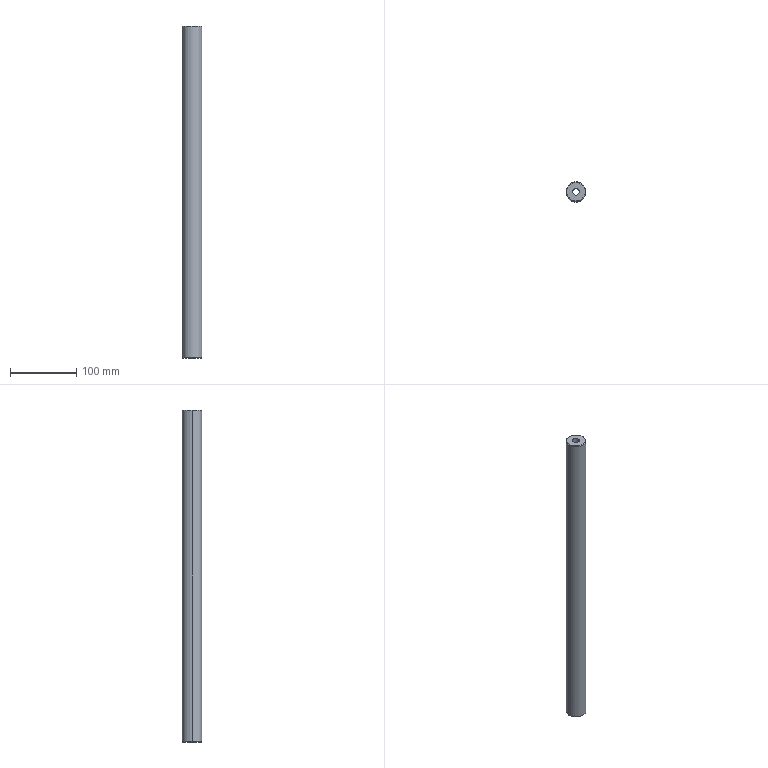Part | SolidWorks | features BaseBody 1 | 1 solid | 10 faces | box 30 x 30 x 500 mm | volume 312481 mm3 | cone 4 | cylinder 4 | plane 2 | commonest cylinder face diameters 10.2 x2 30 x2
STEP:
#1=CARTESIAN_POINT('',(14.,0.,500.));
#2=VERTEX_POINT('',#1);
#3=CARTESIAN_POINT('',(-14.,0.,500.));
#4=VERTEX_POINT('',#3);
#5=CARTESIAN_POINT('',(0.,0.,500.));
#6=DIRECTION('',(0.,0.,1.));
#7=DIRECTION('',(-1.,0.,0.));
#8=AXIS2_PLACEMENT_3D('',#5,#6,#7);
#9=CIRCLE('',#8,14.);
#10=EDGE_CURVE('',#2,#4,#9,.T.);
#11=ORIENTED_EDGE('',*,*,#10,.F.);
#12=CARTESIAN_POINT('',(15.,0.,499.));
#13=VERTEX_POINT('',#12);
#14=CARTESIAN_POINT('',(14.,0.,500.));
#15=DIRECTION('',(0.7071,0.,-0.7071));
#16=VECTOR('',#15,1000.);
#17=LINE('',#14,#16);
#18=EDGE_CURVE('',#2,#13,#17,.T.);
#19=ORIENTED_EDGE('',*,*,#18,.T.);
#20=CARTESIAN_POINT('',(-15.,0.,499.));
#21=VERTEX_POINT('',#20);
#22=CARTESIAN_POINT('',(0.,0.,499.));
#23=DIRECTION('',(0.,0.,-1.));
#24=DIRECTION('',(-1.,0.,0.));
#25=AXIS2_PLACEMENT_3D('',#22,#23,#24);
#26=CIRCLE('',#25,15.);
#27=EDGE_CURVE('',#21,#13,#26,.T.);
#28=ORIENTED_EDGE('',*,*,#27,.F.);
#29=CARTESIAN_POINT('',(-14.,0.,500.));
#30=DIRECTION('',(-0.7071,0.,-0.7071));
#31=VECTOR('',#30,1000.);
#32=LINE('',#29,#31);
#33=EDGE_CURVE('',#4,#21,#32,.T.);
#34=ORIENTED_EDGE('',*,*,#33,.F.);
#35=EDGE_LOOP('',(#11,#19,#28,#34));
#36=FACE_OUTER_BOUND('',#35,.T.);
#37=CARTESIAN_POINT('',(0.,0.,500.));
#38=DIRECTION('',(0.,0.,-1.));
#39=DIRECTION('',(-1.,0.,0.));
#40=AXIS2_PLACEMENT_3D('',#37,#38,#39);
#41=CONICAL_SURFACE('',#40,14.,0.7854);
#42=ADVANCED_FACE('',(#36),#41,.T.);
#43=ORIENTED_EDGE('',*,*,#27,.T.);
#44=CARTESIAN_POINT('',(15.,0.,1.));
#45=VERTEX_POINT('',#44);
#46=CARTESIAN_POINT('',(15.,0.,499.));
#47=DIRECTION('',(0.,0.,-1.));
#48=VECTOR('',#47,1000.);
#49=LINE('',#46,#48);
#50=EDGE_CURVE('',#13,#45,#49,.T.);
#51=ORIENTED_EDGE('',*,*,#50,.T.);
#52=CARTESIAN_POINT('',(-15.,0.,1.));
#53=VERTEX_POINT('',#52);
#54=CARTESIAN_POINT('',(0.,0.,1.));
#55=DIRECTION('',(0.,0.,-1.));
#56=DIRECTION('',(-1.,0.,0.));
#57=AXIS2_PLACEMENT_3D('',#54,#55,#56);
#58=CIRCLE('',#57,15.);
#59=EDGE_CURVE('',#53,#45,#58,.T.);
#60=ORIENTED_EDGE('',*,*,#59,.F.);
#61=CARTESIAN_POINT('',(-15.,0.,499.));
#62=DIRECTION('',(0.,0.,-1.));
#63=VECTOR('',#62,1000.);
#64=LINE('',#61,#63);
#65=EDGE_CURVE('',#21,#53,#64,.T.);
#66=ORIENTED_EDGE('',*,*,#65,.F.);
#67=EDGE_LOOP('',(#43,#51,#60,#66));
#68=FACE_OUTER_BOUND('',#67,.T.);
#69=CARTESIAN_POINT('',(0.,0.,499.));
#70=DIRECTION('',(0.,0.,-1.));
#71=DIRECTION('',(-1.,0.,0.));
#72=AXIS2_PLACEMENT_3D('',#69,#70,#71);
#73=CYLINDRICAL_SURFACE('',#72,15.);
#74=ADVANCED_FACE('',(#68),#73,.T.);
#75=CARTESIAN_POINT('',(5.1,0.,0.));
#76=VERTEX_POINT('',#75);
#77=CARTESIAN_POINT('',(-5.1,0.,0.));
#78=VERTEX_POINT('',#77);
#79=CARTESIAN_POINT('',(0.,0.,0.));
#80=DIRECTION('',(0.,0.,-1.));
#81=DIRECTION('',(1.,0.,0.));
#82=AXIS2_PLACEMENT_3D('',#79,#80,#81);
#83=CIRCLE('',#82,5.1);
#84=EDGE_CURVE('',#76,#78,#83,.T.);
#85=ORIENTED_EDGE('',*,*,#84,.T.);
#86=CARTESIAN_POINT('',(-5.1,0.,500.));
#87=VERTEX_POINT('',#86);
#88=CARTESIAN_POINT('',(-5.1,0.,0.));
#89=DIRECTION('',(0.,0.,1.));
#90=VECTOR('',#89,1000.);
#91=LINE('',#88,#90);
#92=EDGE_CURVE('',#78,#87,#91,.T.);
#93=ORIENTED_EDGE('',*,*,#92,.T.);
#94=CARTESIAN_POINT('',(5.1,0.,500.));
#95=VERTEX_POINT('',#94);
#96=CARTESIAN_POINT('',(0.,0.,500.));
#97=DIRECTION('',(0.,0.,-1.));
#98=DIRECTION('',(1.,0.,0.));
#99=AXIS2_PLACEMENT_3D('',#96,#97,#98);
#100=CIRCLE('',#99,5.1);
#101=EDGE_CURVE('',#95,#87,#100,.T.);
#102=ORIENTED_EDGE('',*,*,#101,.F.);
#103=CARTESIAN_POINT('',(5.1,0.,0.));
#104=DIRECTION('',(0.,0.,1.));
#105=VECTOR('',#104,1000.);
#106=LINE('',#103,#105);
#107=EDGE_CURVE('',#76,#95,#106,.T.);
#108=ORIENTED_EDGE('',*,*,#107,.F.);
#109=EDGE_LOOP('',(#85,#93,#102,#108));
#110=FACE_OUTER_BOUND('',#109,.T.);
#111=CARTESIAN_POINT('',(0.,0.,0.));
#112=DIRECTION('',(0.,0.,1.));
#113=DIRECTION('',(1.,0.,0.));
#114=AXIS2_PLACEMENT_3D('',#111,#112,#113);
#115=CYLINDRICAL_SURFACE('',#114,5.1);
#116=ADVANCED_FACE('',(#110),#115,.F.);
#117=CARTESIAN_POINT('',(-14.,0.,0.));
#118=VERTEX_POINT('',#117);
#119=CARTESIAN_POINT('',(14.,0.,0.));
#120=VERTEX_POINT('',#119);
#121=CARTESIAN_POINT('',(0.,0.,0.));
#122=DIRECTION('',(0.,0.,-1.));
#123=DIRECTION('',(1.,0.,0.));
#124=AXIS2_PLACEMENT_3D('',#121,#122,#123);
#125=CIRCLE('',#124,14.);
#126=EDGE_CURVE('',#118,#120,#125,.T.);
#127=ORIENTED_EDGE('',*,*,#126,.F.);
#128=CARTESIAN_POINT('',(-14.,0.,0.));
#129=DIRECTION('',(-0.7071,0.,0.7071));
#130=VECTOR('',#129,1000.);
#131=LINE('',#128,#130);
#132=EDGE_CURVE('',#118,#53,#131,.T.);
#133=ORIENTED_EDGE('',*,*,#132,.T.);
#134=ORIENTED_EDGE('',*,*,#59,.T.);
#135=CARTESIAN_POINT('',(14.,0.,0.));
#136=DIRECTION('',(0.7071,0.,0.7071));
#137=VECTOR('',#136,1000.);
#138=LINE('',#135,#137);
#139=EDGE_CURVE('',#120,#45,#138,.T.);
#140=ORIENTED_EDGE('',*,*,#139,.F.);
#141=EDGE_LOOP('',(#127,#133,#134,#140));
#142=FACE_OUTER_BOUND('',#141,.T.);
#143=CARTESIAN_POINT('',(0.,0.,0.));
#144=DIRECTION('',(0.,0.,1.));
#145=DIRECTION('',(1.,0.,0.));
#146=AXIS2_PLACEMENT_3D('',#143,#144,#145);
#147=CONICAL_SURFACE('',#146,14.,0.7854);
#148=ADVANCED_FACE('',(#142),#147,.T.);
#149=ORIENTED_EDGE('',*,*,#18,.F.);
#150=CARTESIAN_POINT('',(0.,0.,500.));
#151=DIRECTION('',(0.,0.,1.));
#152=DIRECTION('',(-1.,0.,0.));
#153=AXIS2_PLACEMENT_3D('',#150,#151,#152);
#154=CIRCLE('',#153,14.);
#155=EDGE_CURVE('',#4,#2,#154,.T.);
#156=ORIENTED_EDGE('',*,*,#155,.F.);
#157=ORIENTED_EDGE('',*,*,#33,.T.);
#158=CARTESIAN_POINT('',(0.,0.,499.));
#159=DIRECTION('',(0.,0.,-1.));
#160=DIRECTION('',(-1.,0.,0.));
#161=AXIS2_PLACEMENT_3D('',#158,#159,#160);
#162=CIRCLE('',#161,15.);
#163=EDGE_CURVE('',#13,#21,#162,.T.);
#164=ORIENTED_EDGE('',*,*,#163,.F.);
#165=EDGE_LOOP('',(#149,#156,#157,#164));
#166=FACE_OUTER_BOUND('',#165,.T.);
#167=CARTESIAN_POINT('',(0.,0.,500.));
#168=DIRECTION('',(0.,0.,-1.));
#169=DIRECTION('',(-1.,0.,0.));
#170=AXIS2_PLACEMENT_3D('',#167,#168,#169);
#171=CONICAL_SURFACE('',#170,14.,0.7854);
#172=ADVANCED_FACE('',(#166),#171,.T.);
#173=ORIENTED_EDGE('',*,*,#101,.T.);
#174=CARTESIAN_POINT('',(0.,0.,500.));
#175=DIRECTION('',(0.,0.,-1.));
#176=DIRECTION('',(1.,0.,0.));
#177=AXIS2_PLACEMENT_3D('',#174,#175,#176);
#178=CIRCLE('',#177,5.1);
#179=EDGE_CURVE('',#87,#95,#178,.T.);
#180=ORIENTED_EDGE('',*,*,#179,.T.);
#181=EDGE_LOOP('',(#173,#180));
#182=FACE_BOUND('',#181,.T.);
#183=ORIENTED_EDGE('',*,*,#155,.T.);
#184=ORIENTED_EDGE('',*,*,#10,.T.);
#185=EDGE_LOOP('',(#183,#184));
#186=FACE_OUTER_BOUND('',#185,.T.);
#187=CARTESIAN_POINT('',(-14.168,-14.168,500.));
#188=DIRECTION('',(0.,0.,1.));
#189=DIRECTION('',(1.,0.,0.));
#190=AXIS2_PLACEMENT_3D('',#187,#188,#189);
#191=PLANE('',#190);
#192=ADVANCED_FACE('',(#182,#186),#191,.T.);
#193=ORIENTED_EDGE('',*,*,#50,.F.);
#194=ORIENTED_EDGE('',*,*,#163,.T.);
#195=ORIENTED_EDGE('',*,*,#65,.T.);
#196=CARTESIAN_POINT('',(0.,0.,1.));
#197=DIRECTION('',(0.,0.,-1.));
#198=DIRECTION('',(-1.,0.,0.));
#199=AXIS2_PLACEMENT_3D('',#196,#197,#198);
#200=CIRCLE('',#199,15.);
#201=EDGE_CURVE('',#45,#53,#200,.T.);
#202=ORIENTED_EDGE('',*,*,#201,.F.);
#203=EDGE_LOOP('',(#193,#194,#195,#202));
#204=FACE_OUTER_BOUND('',#203,.T.);
#205=CARTESIAN_POINT('',(0.,0.,499.));
#206=DIRECTION('',(0.,0.,-1.));
#207=DIRECTION('',(-1.,0.,0.));
#208=AXIS2_PLACEMENT_3D('',#205,#206,#207);
#209=CYLINDRICAL_SURFACE('',#208,15.);
#210=ADVANCED_FACE('',(#204),#209,.T.);
#211=ORIENTED_EDGE('',*,*,#92,.F.);
#212=CARTESIAN_POINT('',(0.,0.,0.));
#213=DIRECTION('',(0.,0.,-1.));
#214=DIRECTION('',(1.,0.,0.));
#215=AXIS2_PLACEMENT_3D('',#212,#213,#214);
#216=CIRCLE('',#215,5.1);
#217=EDGE_CURVE('',#78,#76,#216,.T.);
#218=ORIENTED_EDGE('',*,*,#217,.T.);
#219=ORIENTED_EDGE('',*,*,#107,.T.);
#220=ORIENTED_EDGE('',*,*,#179,.F.);
#221=EDGE_LOOP('',(#211,#218,#219,#220));
#222=FACE_OUTER_BOUND('',#221,.T.);
#223=CARTESIAN_POINT('',(0.,0.,0.));
#224=DIRECTION('',(0.,0.,1.));
#225=DIRECTION('',(1.,0.,0.));
#226=AXIS2_PLACEMENT_3D('',#223,#224,#225);
#227=CYLINDRICAL_SURFACE('',#226,5.1);
#228=ADVANCED_FACE('',(#222),#227,.F.);
#229=ORIENTED_EDGE('',*,*,#132,.F.);
#230=CARTESIAN_POINT('',(0.,0.,0.));
#231=DIRECTION('',(0.,0.,-1.));
#232=DIRECTION('',(1.,0.,0.));
#233=AXIS2_PLACEMENT_3D('',#230,#231,#232);
#234=CIRCLE('',#233,14.);
#235=EDGE_CURVE('',#120,#118,#234,.T.);
#236=ORIENTED_EDGE('',*,*,#235,.F.);
#237=ORIENTED_EDGE('',*,*,#139,.T.);
#238=ORIENTED_EDGE('',*,*,#201,.T.);
#239=EDGE_LOOP('',(#229,#236,#237,#238));
#240=FACE_OUTER_BOUND('',#239,.T.);
#241=CARTESIAN_POINT('',(0.,0.,0.));
#242=DIRECTION('',(0.,0.,1.));
#243=DIRECTION('',(1.,0.,0.));
#244=AXIS2_PLACEMENT_3D('',#241,#242,#243);
#245=CONICAL_SURFACE('',#244,14.,0.7854);
#246=ADVANCED_FACE('',(#240),#245,.T.);
#247=ORIENTED_EDGE('',*,*,#84,.F.);
#248=ORIENTED_EDGE('',*,*,#217,.F.);
#249=EDGE_LOOP('',(#247,#248));
#250=FACE_BOUND('',#249,.T.);
#251=ORIENTED_EDGE('',*,*,#235,.T.);
#252=ORIENTED_EDGE('',*,*,#126,.T.);
#253=EDGE_LOOP('',(#251,#252));
#254=FACE_OUTER_BOUND('',#253,.T.);
#255=CARTESIAN_POINT('',(-14.168,-14.168,0.));
#256=DIRECTION('',(0.,0.,1.));
#257=DIRECTION('',(1.,0.,0.));
#258=AXIS2_PLACEMENT_3D('',#255,#256,#257);
#259=PLANE('',#258);
#260=ADVANCED_FACE('',(#250,#254),#259,.F.);
#261=CLOSED_SHELL('',(#42,#74,#116,#148,#172,#192,#210,#228,#246,#260));
#262=MANIFOLD_SOLID_BREP('',#261);
#263=CARTESIAN_POINT('',(0.,0.,0.));
#264=DIRECTION('',(0.,0.,1.));
#265=DIRECTION('',(1.,0.,0.));
#266=AXIS2_PLACEMENT_3D('',#263,#264,#265);
#267=(LENGTH_UNIT()NAMED_UNIT(*)SI_UNIT(.MILLI.,.METRE.));
#268=UNCERTAINTY_MEASURE_WITH_UNIT(LENGTH_MEASURE(0.00001),#267,'','');
#269=(NAMED_UNIT(*)PLANE_ANGLE_UNIT()SI_UNIT($,.RADIAN.));
#270=(NAMED_UNIT(*)SI_UNIT($,.STERADIAN.)SOLID_ANGLE_UNIT());
#271=(GEOMETRIC_REPRESENTATION_CONTEXT(3)GLOBAL_UNCERTAINTY_ASSIGNED_CONTEXT((#268))GLOBAL_UNIT_ASSIGNED_CONTEXT((#267,#269,#270))REPRESENTATION_CONTEXT('',''));
#272=ADVANCED_BREP_SHAPE_REPRESENTATION('',(#262,#266),#271);